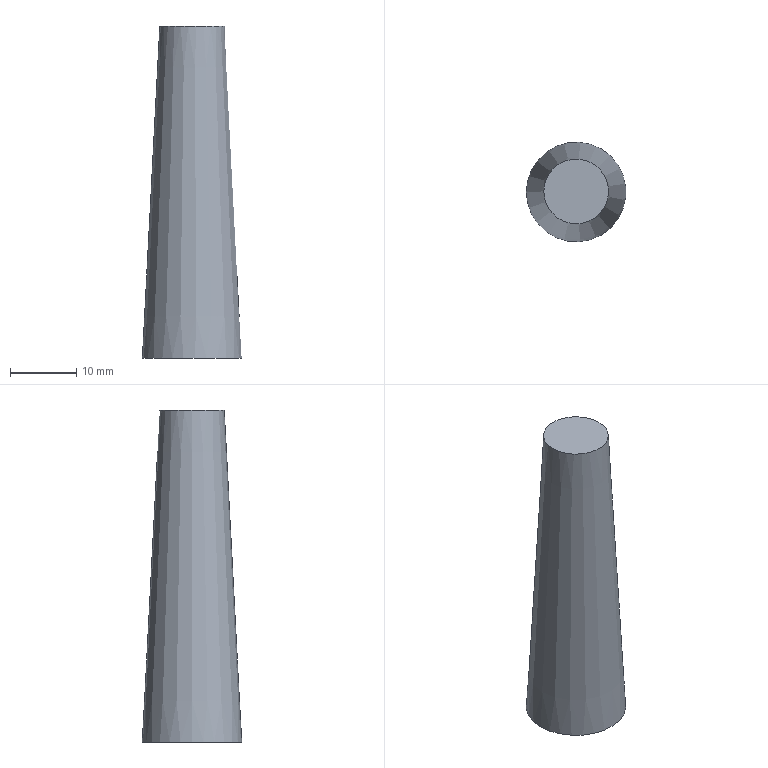Part | STEP file | Upper_shell_sub | 1 solid | 3 faces | box 15 x 15 x 50 mm | volume 6108 mm3 | plane 2 | cone 1
STEP:
#1=CARTESIAN_POINT('',(0.,0.,0.));
#2=DIRECTION('',(0.,0.,1.));
#3=DIRECTION('',(1.,0.,0.));
#4=AXIS2_PLACEMENT_3D('',#1,#2,#3);
#5=CARTESIAN_POINT('',(-57.947,40.989,260.));
#6=VERTEX_POINT('',#5);
#7=CARTESIAN_POINT('',(-50.447,40.989,260.));
#8=DIRECTION('',(0.,0.,1.));
#9=DIRECTION('',(-1.,0.,0.));
#10=AXIS2_PLACEMENT_3D('',#7,#8,#9);
#11=CIRCLE('',#10,7.5);
#12=CARTESIAN_POINT('',(-50.447,40.989,260.));
#13=DIRECTION('',(0.,0.,1.));
#14=DIRECTION('',(-1.,0.,0.));
#15=AXIS2_PLACEMENT_3D('',#12,#13,#14);
#16=PLANE('',#15);
#17=CARTESIAN_POINT('',(0.,0.));
#18=DIRECTION('',(1.,0.));
#19=AXIS2_PLACEMENT_2D('',#17,#18);
#20=CIRCLE('',#19,7.5);
#21=(GEOMETRIC_REPRESENTATION_CONTEXT(2)PARAMETRIC_REPRESENTATION_CONTEXT()REPRESENTATION_CONTEXT('',''));
#22=DEFINITIONAL_REPRESENTATION('',(#20),#21);
#23=PCURVE('',#16,#22);
#24=CARTESIAN_POINT('',(-50.447,40.989,260.));
#25=DIRECTION('',(0.,0.,-1.));
#26=DIRECTION('',(-1.,0.,0.));
#27=AXIS2_PLACEMENT_3D('',#24,#25,#26);
#28=CONICAL_SURFACE('',#27,7.5,0.05236);
#29=CARTESIAN_POINT('',(6.283,0.));
#30=DIRECTION('',(-1.,0.));
#31=VECTOR('',#30,1.);
#32=LINE('',#29,#31);
#33=(GEOMETRIC_REPRESENTATION_CONTEXT(2)PARAMETRIC_REPRESENTATION_CONTEXT()REPRESENTATION_CONTEXT('',''));
#34=DEFINITIONAL_REPRESENTATION('',(#32),#33);
#35=PCURVE('',#28,#34);
#36=SURFACE_CURVE('',#11,(#23,#35),.PCURVE_S1.);
#37=EDGE_CURVE('',#6,#6,#36,.T.);
#38=ORIENTED_EDGE('',*,*,#37,.F.);
#39=EDGE_LOOP('',(#38));
#40=FACE_BOUND('',#39,.T.);
#41=ADVANCED_FACE('',(#40),#16,.F.);
#42=CARTESIAN_POINT('',(-55.327,40.989,310.));
#43=VERTEX_POINT('',#42);
#44=CARTESIAN_POINT('',(-50.447,40.989,310.));
#45=DIRECTION('',(0.,0.,-1.));
#46=DIRECTION('',(-1.,0.,0.));
#47=AXIS2_PLACEMENT_3D('',#44,#45,#46);
#48=CIRCLE('',#47,4.88);
#49=CARTESIAN_POINT('',(-50.447,40.989,310.));
#50=DIRECTION('',(0.,0.,1.));
#51=DIRECTION('',(-1.,0.,0.));
#52=AXIS2_PLACEMENT_3D('',#49,#50,#51);
#53=PLANE('',#52);
#54=CARTESIAN_POINT('',(4.88,0.));
#55=CARTESIAN_POINT('',(4.88,-8.452));
#56=CARTESIAN_POINT('',(-2.44,-4.226));
#57=CARTESIAN_POINT('',(-9.759,0.));
#58=CARTESIAN_POINT('',(-2.44,4.226));
#59=CARTESIAN_POINT('',(4.88,8.452));
#60=CARTESIAN_POINT('',(4.88,0.));
#61=(BOUNDED_CURVE()B_SPLINE_CURVE(2,(#54,#55,#56,#57,#58,#59,#60),.UNSPECIFIED.,.T.,.F.)B_SPLINE_CURVE_WITH_KNOTS((1,2,2,2,2,1),(-2.094,0.,2.094,4.189,6.283,8.378),.UNSPECIFIED.)CURVE()GEOMETRIC_REPRESENTATION_ITEM()RATIONAL_B_SPLINE_CURVE((1.,0.5,1.,0.5,1.,0.5,1.))REPRESENTATION_ITEM(''));
#62=(GEOMETRIC_REPRESENTATION_CONTEXT(2)PARAMETRIC_REPRESENTATION_CONTEXT()REPRESENTATION_CONTEXT('',''));
#63=DEFINITIONAL_REPRESENTATION('',(#61),#62);
#64=PCURVE('',#53,#63);
#65=CARTESIAN_POINT('',(0.,-50.));
#66=DIRECTION('',(1.,0.));
#67=VECTOR('',#66,1.);
#68=LINE('',#65,#67);
#69=(GEOMETRIC_REPRESENTATION_CONTEXT(2)PARAMETRIC_REPRESENTATION_CONTEXT()REPRESENTATION_CONTEXT('',''));
#70=DEFINITIONAL_REPRESENTATION('',(#68),#69);
#71=PCURVE('',#28,#70);
#72=SURFACE_CURVE('',#48,(#64,#71),.PCURVE_S1.);
#73=EDGE_CURVE('',#43,#43,#72,.T.);
#74=ORIENTED_EDGE('',*,*,#73,.F.);
#75=EDGE_LOOP('',(#74));
#76=FACE_BOUND('',#75,.T.);
#77=ADVANCED_FACE('',(#76),#53,.T.);
#78=ORIENTED_EDGE('',*,*,#37,.T.);
#79=CARTESIAN_POINT('',(-55.327,40.989,310.));
#80=CARTESIAN_POINT('',(-57.947,40.989,260.));
#81=B_SPLINE_CURVE_WITH_KNOTS('',1,(#79,#80),.UNSPECIFIED.,.F.,.F.,(2,2),(-50.069,0.),.PIECEWISE_BEZIER_KNOTS.);
#82=CARTESIAN_POINT('',(0.,0.));
#83=DIRECTION('',(0.,1.));
#84=VECTOR('',#83,1.);
#85=LINE('',#82,#84);
#86=(GEOMETRIC_REPRESENTATION_CONTEXT(2)PARAMETRIC_REPRESENTATION_CONTEXT()REPRESENTATION_CONTEXT('',''));
#87=DEFINITIONAL_REPRESENTATION('',(#85),#86);
#88=PCURVE('',#28,#87);
#89=CARTESIAN_POINT('',(6.283,0.));
#90=DIRECTION('',(0.,1.));
#91=VECTOR('',#90,1.);
#92=LINE('',#89,#91);
#93=(GEOMETRIC_REPRESENTATION_CONTEXT(2)PARAMETRIC_REPRESENTATION_CONTEXT()REPRESENTATION_CONTEXT('',''));
#94=DEFINITIONAL_REPRESENTATION('',(#92),#93);
#95=PCURVE('',#28,#94);
#96=SEAM_CURVE('',#81,(#88,#95),.PCURVE_S1.);
#97=EDGE_CURVE('',#43,#6,#96,.T.);
#98=ORIENTED_EDGE('',*,*,#97,.F.);
#99=ORIENTED_EDGE('',*,*,#73,.T.);
#100=ORIENTED_EDGE('',*,*,#97,.T.);
#101=EDGE_LOOP('',(#78,#98,#99,#100));
#102=FACE_BOUND('',#101,.T.);
#103=ADVANCED_FACE('',(#102),#28,.T.);
#104=CLOSED_SHELL('',(#41,#77,#103));
#105=MANIFOLD_SOLID_BREP('',#104);
#106=(LENGTH_UNIT()NAMED_UNIT(*)SI_UNIT(.MILLI.,.METRE.));
#107=UNCERTAINTY_MEASURE_WITH_UNIT(LENGTH_MEASURE(0.0000001),#106,'','');
#108=(NAMED_UNIT(*)PLANE_ANGLE_UNIT()SI_UNIT($,.RADIAN.));
#109=(NAMED_UNIT(*)SI_UNIT($,.STERADIAN.)SOLID_ANGLE_UNIT());
#110=(GEOMETRIC_REPRESENTATION_CONTEXT(3)GLOBAL_UNCERTAINTY_ASSIGNED_CONTEXT((#107))GLOBAL_UNIT_ASSIGNED_CONTEXT((#106,#108,#109))REPRESENTATION_CONTEXT('',''));
#111=ADVANCED_BREP_SHAPE_REPRESENTATION('',(#4,#105),#110);